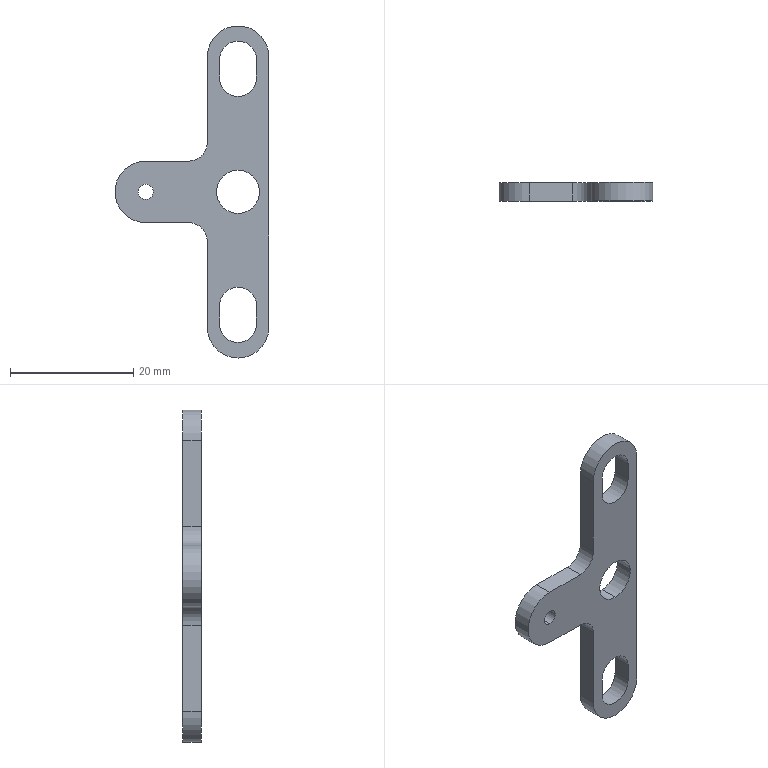Part | STEP file | 0246_213_Plate | 1 solid | 27 faces | box 25 x 3 x 54 mm | volume 1577 mm3 | cylinder 16 | plane 11 | commonest cylinder face diameters 6 x8 10 x4 2.5 x2 7 x2